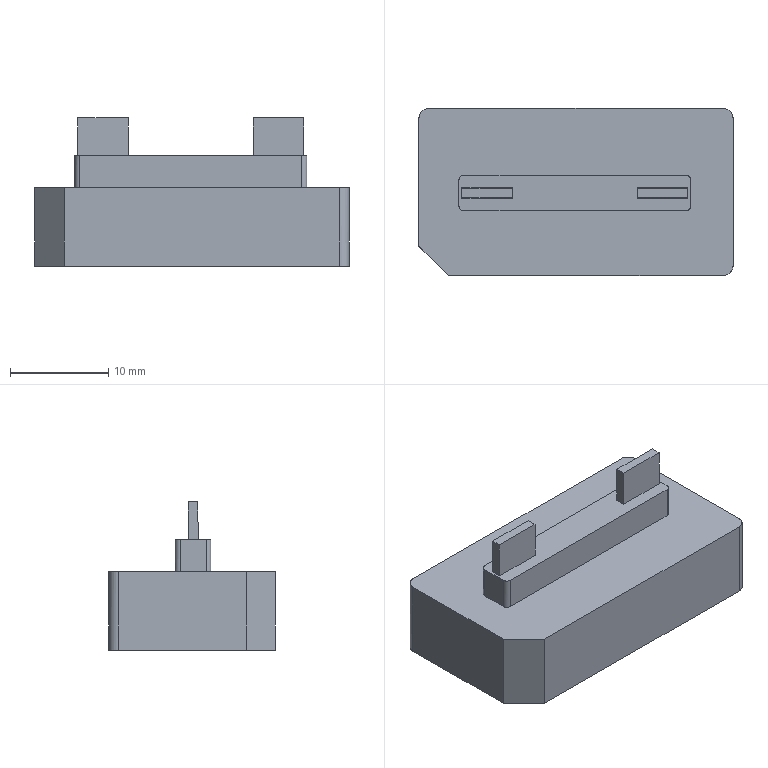CAM job | PowerMill | 3-axis milling, other | part box 32 x 17 x 15.109 mm
Tools:
number,name,type,diameter,tip_radius,length,cutting_length,overhang,flutes,holder,toolpaths_using
1,D10C_1_1,end_mill,10.0,0.0,60.0,,15.56,1,D42L35,6
3,D10_1_1,end_mill,10.0,0.0,60.0,,15.28,1,D42L35,8
10,D3_1_1,end_mill,3.0,0.0,30.0,,7.28,1,D42L35,2
13,Text_D4_1_1,taper_spherical,4.0,0.3,60.0,,7.36,1,D42L35,2
10,D3_2_1,end_mill,3.0,0.0,30.0,,7.2,1,D42L35,2
Operations:
program,toolpath,strategy,tool,tool_number,tool_diameter,tip_radius,flutes,spindle_rpm,feed_cut,surface_speed_m_min_computed,feed_per_tooth_computed,tolerance,thickness,stepover,stepdown,cut_length,cut_time_min,total_time_min,workplane
08-0613-3-F,精公开粗01-扫面平行-D10C,raster_area_clear,D10C_1_1,1,10.0,0.0,1.0,8000.0,10000.0,251.33,1.25,0.03,0.28,6.0,1.0,210.36,0.021,0.0268,
08-0613-3-F,精公开粗01-外形偏置-D10C,offset_area_clear,D10C_1_1,1,10.0,0.0,1.0,8000.0,10000.0,251.33,1.25,0.03,0.28,6.0,1.0,3933.122,0.393,0.4401,
08-0613-3-F,精公开粗01-基准台等高-D10C,constantz,D10C_1_1,1,10.0,0.0,1.0,8000.0,10000.0,251.33,1.25,0.03,0.07,5.0,0.4,2789.059,0.279,0.2878,
08-0613-3-F,精公基准台01-平坦面偏置-D10,offset_area_clear,D10_1_1,3,10.0,0.0,1.0,8500.0,600.0,267.04,0.0706,0.005,0.38,5.0,1.0,141.709,0.236,0.3008,
08-0613-3-F,精公基准台01-基准面偏置-D10,offset_area_clear,D10_1_1,3,10.0,0.0,1.0,8500.0,600.0,267.04,0.0706,0.005,0.38,5.0,1.0,96.75,0.161,0.1793,
08-0613-3-F,精公基准台01-外形侧光-D10,profile_area_clear,D10_1_1,3,10.0,0.0,1.0,8500.0,600.0,267.04,0.0706,0.005,-0.07,0.08,1.0,169.673,0.283,0.3025,
08-0613-3-F,精公基准台01-基准台侧光-D10,profile_area_clear,D10_1_1,3,10.0,0.0,1.0,8500.0,600.0,267.04,0.0706,0.005,0.0,0.08,1.0,253.233,0.422,0.4855,
08-0613-3-F,精公精光01-等高-D3,constantz,D3_1_1,10,3.0,0.0,1.0,18000.0,2000.0,169.65,0.1111,0.005,-0.075,5.0,0.03,12214.312,6.107,6.119,
08-0613-3-F,精公精光01-平坦面偏置-D3,offset_area_clear,D3_1_1,10,3.0,0.0,1.0,18000.0,600.0,169.65,0.0333,0.005,0.375,1.5,1.0,115.514,0.193,0.2294,
08-0613-3-F,精公刻字01-刻字-Text_D4,pattern,Text_D4_1_1,13,4.0,0.3,1.0,15000.0,1000.0,188.5,0.0667,0.005,0.0,5.0,1.0,60.977,0.061,0.0793,
08-0613-3-R,粗公开粗01-扫面平行-D10C,raster_area_clear,D10C_1_1,1,10.0,0.0,1.0,8000.0,10000.0,251.33,1.25,0.03,0.2,6.0,1.0,209.4,0.021,0.0267,
08-0613-3-R,粗公开粗01-外形偏置-D10C,offset_area_clear,D10C_1_1,1,10.0,0.0,1.0,8000.0,10000.0,251.33,1.25,0.03,0.2,6.0,1.0,3910.653,0.391,0.4378,
08-0613-3-R,粗公开粗01-基准台等高-D10C,constantz,D10C_1_1,1,10.0,0.0,1.0,8000.0,10000.0,251.33,1.25,0.03,0.07,5.0,0.4,2789.059,0.279,0.2878,
08-0613-3-R,粗公基准台01-平坦面偏置-D10,offset_area_clear,D10_1_1,3,10.0,0.0,1.0,8500.0,600.0,267.04,0.0706,0.01,0.3,5.0,1.0,139.335,0.232,0.3052,
08-0613-3-R,粗公基准台01-基准面偏置-D10,offset_area_clear,D10_1_1,3,10.0,0.0,1.0,8500.0,600.0,267.04,0.0706,0.01,0.3,5.0,1.0,96.22,0.16,0.1784,
08-0613-3-R,粗公基准台01-外形侧光-D10,profile_area_clear,D10_1_1,3,10.0,0.0,1.0,8500.0,600.0,267.04,0.0706,0.01,-0.15,0.08,1.0,168.659,0.281,0.3008,
08-0613-3-R,粗公基准台01-基准台侧光-D10,profile_area_clear,D10_1_1,3,10.0,0.0,1.0,8500.0,600.0,267.04,0.0706,0.01,0.0,0.08,1.0,253.217,0.422,0.4854,
08-0613-3-R,粗公精光01-等高-D3,constantz,D3_2_1,10,3.0,0.0,1.0,18000.0,2000.0,169.65,0.1111,0.01,-0.155,5.0,0.036,9876.528,4.938,4.95,
08-0613-3-R,粗公精光01-平坦面偏置-D3,offset_area_clear,D3_2_1,10,3.0,0.0,1.0,18000.0,600.0,169.65,0.0333,0.01,0.295,1.5,1.0,113.592,0.189,0.2267,
08-0613-3-R,粗公刻字01-刻字-Text_D4,pattern,Text_D4_1_1,13,4.0,0.3,1.0,15000.0,1000.0,188.5,0.0667,0.01,0.0,5.0,1.0,60.209,0.06,0.0786,